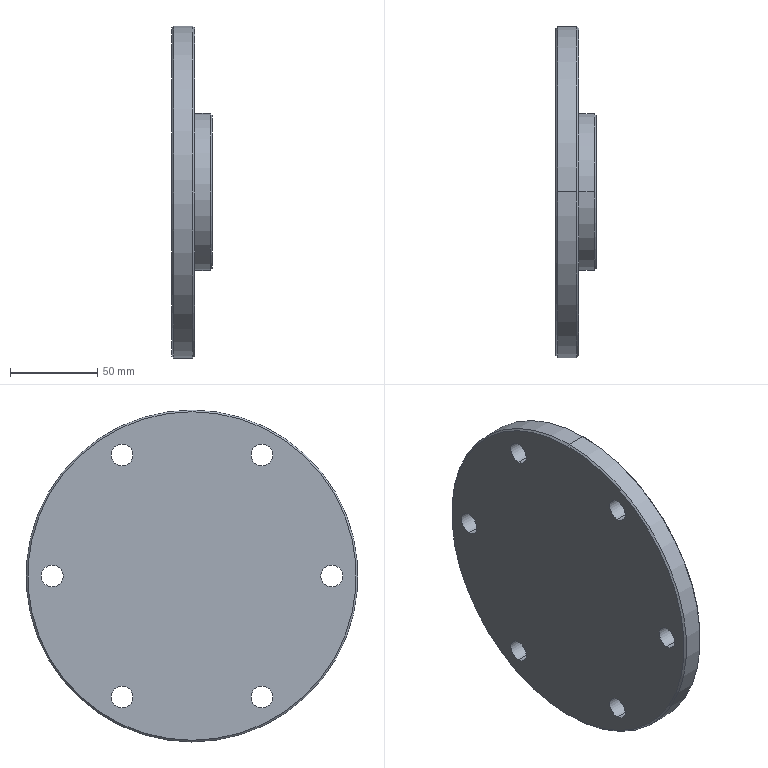Part | SolidWorks | features Chamfer 1, CirPattern 1, ICE 1, Revolution 1 | 1 solid | 30 faces | box 23 x 190 x 190 mm | volume 393528 mm3 | cylinder 18 | cone 8 | plane 4 | commonest cylinder face diameters 12.5 x12 60 x2 90 x2 190 x2
STEP:
#1=CARTESIAN_POINT('',(13.,0.,-94.));
#2=VERTEX_POINT('',#1);
#3=CARTESIAN_POINT('',(13.,0.,94.));
#4=VERTEX_POINT('',#3);
#5=CARTESIAN_POINT('',(13.,0.,0.));
#6=DIRECTION('',(1.,0.,0.));
#7=DIRECTION('',(0.,0.,1.));
#8=AXIS2_PLACEMENT_3D('',#5,#6,#7);
#9=CIRCLE('',#8,94.);
#10=EDGE_CURVE('',#2,#4,#9,.T.);
#11=ORIENTED_EDGE('',*,*,#10,.F.);
#12=CARTESIAN_POINT('',(12.,0.,-95.));
#13=VERTEX_POINT('',#12);
#14=CARTESIAN_POINT('',(12.,0.,-95.));
#15=DIRECTION('',(-0.7071,0.,-0.7071));
#16=VECTOR('',#15,1000.);
#17=LINE('',#14,#16);
#18=EDGE_CURVE('',#2,#13,#17,.T.);
#19=ORIENTED_EDGE('',*,*,#18,.T.);
#20=CARTESIAN_POINT('',(12.,0.,95.));
#21=VERTEX_POINT('',#20);
#22=CARTESIAN_POINT('',(12.,0.,0.));
#23=DIRECTION('',(-1.,0.,0.));
#24=DIRECTION('',(0.,0.,1.));
#25=AXIS2_PLACEMENT_3D('',#22,#23,#24);
#26=CIRCLE('',#25,95.);
#27=EDGE_CURVE('',#21,#13,#26,.T.);
#28=ORIENTED_EDGE('',*,*,#27,.F.);
#29=CARTESIAN_POINT('',(12.,0.,95.));
#30=DIRECTION('',(-0.7071,0.,0.7071));
#31=VECTOR('',#30,1000.);
#32=LINE('',#29,#31);
#33=EDGE_CURVE('',#4,#21,#32,.T.);
#34=ORIENTED_EDGE('',*,*,#33,.F.);
#35=EDGE_LOOP('',(#11,#19,#28,#34));
#36=FACE_OUTER_BOUND('',#35,.T.);
#37=CARTESIAN_POINT('',(12.,0.,0.));
#38=DIRECTION('',(-1.,0.,0.));
#39=DIRECTION('',(0.,0.,1.));
#40=AXIS2_PLACEMENT_3D('',#37,#38,#39);
#41=CONICAL_SURFACE('',#40,95.,0.7854);
#42=ADVANCED_FACE('',(#36),#41,.T.);
#43=CARTESIAN_POINT('',(0.,0.,94.));
#44=VERTEX_POINT('',#43);
#45=CARTESIAN_POINT('',(0.,0.,-94.));
#46=VERTEX_POINT('',#45);
#47=CARTESIAN_POINT('',(0.,0.,0.));
#48=DIRECTION('',(-1.,0.,0.));
#49=DIRECTION('',(0.,0.,-1.));
#50=AXIS2_PLACEMENT_3D('',#47,#48,#49);
#51=CIRCLE('',#50,94.);
#52=EDGE_CURVE('',#44,#46,#51,.T.);
#53=ORIENTED_EDGE('',*,*,#52,.F.);
#54=CARTESIAN_POINT('',(1.,0.,95.));
#55=VERTEX_POINT('',#54);
#56=CARTESIAN_POINT('',(0.,0.,94.));
#57=DIRECTION('',(0.7071,0.,0.7071));
#58=VECTOR('',#57,1000.);
#59=LINE('',#56,#58);
#60=EDGE_CURVE('',#44,#55,#59,.T.);
#61=ORIENTED_EDGE('',*,*,#60,.T.);
#62=CARTESIAN_POINT('',(1.,0.,-95.));
#63=VERTEX_POINT('',#62);
#64=CARTESIAN_POINT('',(1.,0.,0.));
#65=DIRECTION('',(1.,0.,0.));
#66=DIRECTION('',(0.,0.,-1.));
#67=AXIS2_PLACEMENT_3D('',#64,#65,#66);
#68=CIRCLE('',#67,95.);
#69=EDGE_CURVE('',#63,#55,#68,.T.);
#70=ORIENTED_EDGE('',*,*,#69,.F.);
#71=CARTESIAN_POINT('',(0.,0.,-94.));
#72=DIRECTION('',(0.7071,0.,-0.7071));
#73=VECTOR('',#72,1000.);
#74=LINE('',#71,#73);
#75=EDGE_CURVE('',#46,#63,#74,.T.);
#76=ORIENTED_EDGE('',*,*,#75,.F.);
#77=EDGE_LOOP('',(#53,#61,#70,#76));
#78=FACE_OUTER_BOUND('',#77,.T.);
#79=CARTESIAN_POINT('',(0.,0.,0.));
#80=DIRECTION('',(1.,0.,0.));
#81=DIRECTION('',(0.,0.,-1.));
#82=AXIS2_PLACEMENT_3D('',#79,#80,#81);
#83=CONICAL_SURFACE('',#82,94.,0.7854);
#84=ADVANCED_FACE('',(#78),#83,.T.);
#85=CARTESIAN_POINT('',(23.,0.,-44.));
#86=VERTEX_POINT('',#85);
#87=CARTESIAN_POINT('',(23.,0.,44.));
#88=VERTEX_POINT('',#87);
#89=CARTESIAN_POINT('',(23.,0.,0.));
#90=DIRECTION('',(1.,0.,0.));
#91=DIRECTION('',(0.,0.,1.));
#92=AXIS2_PLACEMENT_3D('',#89,#90,#91);
#93=CIRCLE('',#92,44.);
#94=EDGE_CURVE('',#86,#88,#93,.T.);
#95=ORIENTED_EDGE('',*,*,#94,.F.);
#96=CARTESIAN_POINT('',(22.,0.,-45.));
#97=VERTEX_POINT('',#96);
#98=CARTESIAN_POINT('',(22.,0.,-45.));
#99=DIRECTION('',(-0.7071,0.,-0.7071));
#100=VECTOR('',#99,1000.);
#101=LINE('',#98,#100);
#102=EDGE_CURVE('',#86,#97,#101,.T.);
#103=ORIENTED_EDGE('',*,*,#102,.T.);
#104=CARTESIAN_POINT('',(22.,0.,45.));
#105=VERTEX_POINT('',#104);
#106=CARTESIAN_POINT('',(22.,0.,0.));
#107=DIRECTION('',(-1.,0.,0.));
#108=DIRECTION('',(0.,0.,1.));
#109=AXIS2_PLACEMENT_3D('',#106,#107,#108);
#110=CIRCLE('',#109,45.);
#111=EDGE_CURVE('',#105,#97,#110,.T.);
#112=ORIENTED_EDGE('',*,*,#111,.F.);
#113=CARTESIAN_POINT('',(22.,0.,45.));
#114=DIRECTION('',(-0.7071,0.,0.7071));
#115=VECTOR('',#114,1000.);
#116=LINE('',#113,#115);
#117=EDGE_CURVE('',#88,#105,#116,.T.);
#118=ORIENTED_EDGE('',*,*,#117,.F.);
#119=EDGE_LOOP('',(#95,#103,#112,#118));
#120=FACE_OUTER_BOUND('',#119,.T.);
#121=CARTESIAN_POINT('',(22.,0.,0.));
#122=DIRECTION('',(-1.,0.,0.));
#123=DIRECTION('',(0.,0.,1.));
#124=AXIS2_PLACEMENT_3D('',#121,#122,#123);
#125=CONICAL_SURFACE('',#124,45.,0.7854);
#126=ADVANCED_FACE('',(#120),#125,.T.);
#127=CARTESIAN_POINT('',(22.,0.,30.));
#128=VERTEX_POINT('',#127);
#129=CARTESIAN_POINT('',(22.,0.,-30.));
#130=VERTEX_POINT('',#129);
#131=CARTESIAN_POINT('',(22.,0.,0.));
#132=DIRECTION('',(1.,0.,0.));
#133=DIRECTION('',(0.,0.,1.));
#134=AXIS2_PLACEMENT_3D('',#131,#132,#133);
#135=CIRCLE('',#134,30.);
#136=EDGE_CURVE('',#128,#130,#135,.T.);
#137=ORIENTED_EDGE('',*,*,#136,.F.);
#138=CARTESIAN_POINT('',(23.,0.,31.));
#139=VERTEX_POINT('',#138);
#140=CARTESIAN_POINT('',(23.,0.,31.));
#141=DIRECTION('',(0.7071,0.,0.7071));
#142=VECTOR('',#141,1000.);
#143=LINE('',#140,#142);
#144=EDGE_CURVE('',#128,#139,#143,.T.);
#145=ORIENTED_EDGE('',*,*,#144,.T.);
#146=CARTESIAN_POINT('',(23.,0.,-31.));
#147=VERTEX_POINT('',#146);
#148=CARTESIAN_POINT('',(23.,0.,0.));
#149=DIRECTION('',(-1.,0.,0.));
#150=DIRECTION('',(0.,0.,1.));
#151=AXIS2_PLACEMENT_3D('',#148,#149,#150);
#152=CIRCLE('',#151,31.);
#153=EDGE_CURVE('',#147,#139,#152,.T.);
#154=ORIENTED_EDGE('',*,*,#153,.F.);
#155=CARTESIAN_POINT('',(23.,0.,-31.));
#156=DIRECTION('',(0.7071,0.,-0.7071));
#157=VECTOR('',#156,1000.);
#158=LINE('',#155,#157);
#159=EDGE_CURVE('',#130,#147,#158,.T.);
#160=ORIENTED_EDGE('',*,*,#159,.F.);
#161=EDGE_LOOP('',(#137,#145,#154,#160));
#162=FACE_OUTER_BOUND('',#161,.T.);
#163=CARTESIAN_POINT('',(23.,0.,0.));
#164=DIRECTION('',(1.,0.,0.));
#165=DIRECTION('',(0.,0.,-1.));
#166=AXIS2_PLACEMENT_3D('',#163,#164,#165);
#167=CONICAL_SURFACE('',#166,31.,0.7854);
#168=ADVANCED_FACE('',(#162),#167,.F.);
#169=CARTESIAN_POINT('',(13.,-40.,-75.532));
#170=VERTEX_POINT('',#169);
#171=CARTESIAN_POINT('',(13.,-40.,-63.032));
#172=VERTEX_POINT('',#171);
#173=CARTESIAN_POINT('',(13.,-40.,-69.282));
#174=DIRECTION('',(-1.,0.,0.));
#175=DIRECTION('',(0.,0.,1.));
#176=AXIS2_PLACEMENT_3D('',#173,#174,#175);
#177=CIRCLE('',#176,6.25);
#178=EDGE_CURVE('',#170,#172,#177,.T.);
#179=ORIENTED_EDGE('',*,*,#178,.F.);
#180=CARTESIAN_POINT('',(0.,-40.,-75.532));
#181=VERTEX_POINT('',#180);
#182=CARTESIAN_POINT('',(23.,-40.,-75.532));
#183=DIRECTION('',(-1.,0.,0.));
#184=VECTOR('',#183,1000.);
#185=LINE('',#182,#184);
#186=EDGE_CURVE('',#170,#181,#185,.T.);
#187=ORIENTED_EDGE('',*,*,#186,.T.);
#188=CARTESIAN_POINT('',(0.,-40.,-63.032));
#189=VERTEX_POINT('',#188);
#190=CARTESIAN_POINT('',(0.,-40.,-69.282));
#191=DIRECTION('',(-1.,0.,0.));
#192=DIRECTION('',(0.,0.866,-0.5));
#193=AXIS2_PLACEMENT_3D('',#190,#191,#192);
#194=CIRCLE('',#193,6.25);
#195=EDGE_CURVE('',#181,#189,#194,.T.);
#196=ORIENTED_EDGE('',*,*,#195,.T.);
#197=CARTESIAN_POINT('',(23.,-40.,-63.032));
#198=DIRECTION('',(-1.,0.,0.));
#199=VECTOR('',#198,1000.);
#200=LINE('',#197,#199);
#201=EDGE_CURVE('',#172,#189,#200,.T.);
#202=ORIENTED_EDGE('',*,*,#201,.F.);
#203=EDGE_LOOP('',(#179,#187,#196,#202));
#204=FACE_OUTER_BOUND('',#203,.T.);
#205=CARTESIAN_POINT('',(23.,-40.,-69.282));
#206=DIRECTION('',(-1.,0.,0.));
#207=DIRECTION('',(0.,0.,1.));
#208=AXIS2_PLACEMENT_3D('',#205,#206,#207);
#209=CYLINDRICAL_SURFACE('',#208,6.25);
#210=ADVANCED_FACE('',(#204),#209,.F.);
#211=CARTESIAN_POINT('',(13.,-80.,-6.25));
#212=VERTEX_POINT('',#211);
#213=CARTESIAN_POINT('',(13.,-80.,6.25));
#214=VERTEX_POINT('',#213);
#215=CARTESIAN_POINT('',(13.,-80.,0.));
#216=DIRECTION('',(-1.,0.,0.));
#217=DIRECTION('',(0.,0.,1.));
#218=AXIS2_PLACEMENT_3D('',#215,#216,#217);
#219=CIRCLE('',#218,6.25);
#220=EDGE_CURVE('',#212,#214,#219,.T.);
#221=ORIENTED_EDGE('',*,*,#220,.F.);
#222=CARTESIAN_POINT('',(0.,-80.,-6.25));
#223=VERTEX_POINT('',#222);
#224=CARTESIAN_POINT('',(23.,-80.,-6.25));
#225=DIRECTION('',(-1.,0.,0.));
#226=VECTOR('',#225,1000.);
#227=LINE('',#224,#226);
#228=EDGE_CURVE('',#212,#223,#227,.T.);
#229=ORIENTED_EDGE('',*,*,#228,.T.);
#230=CARTESIAN_POINT('',(0.,-80.,6.25));
#231=VERTEX_POINT('',#230);
#232=CARTESIAN_POINT('',(0.,-80.,0.));
#233=DIRECTION('',(-1.,0.,0.));
#234=DIRECTION('',(0.,0.,-1.));
#235=AXIS2_PLACEMENT_3D('',#232,#233,#234);
#236=CIRCLE('',#235,6.25);
#237=EDGE_CURVE('',#223,#231,#236,.T.);
#238=ORIENTED_EDGE('',*,*,#237,.T.);
#239=CARTESIAN_POINT('',(23.,-80.,6.25));
#240=DIRECTION('',(-1.,0.,0.));
#241=VECTOR('',#240,1000.);
#242=LINE('',#239,#241);
#243=EDGE_CURVE('',#214,#231,#242,.T.);
#244=ORIENTED_EDGE('',*,*,#243,.F.);
#245=EDGE_LOOP('',(#221,#229,#238,#244));
#246=FACE_OUTER_BOUND('',#245,.T.);
#247=CARTESIAN_POINT('',(23.,-80.,0.));
#248=DIRECTION('',(-1.,0.,0.));
#249=DIRECTION('',(0.,0.,1.));
#250=AXIS2_PLACEMENT_3D('',#247,#248,#249);
#251=CYLINDRICAL_SURFACE('',#250,6.25);
#252=ADVANCED_FACE('',(#246),#251,.F.);
#253=CARTESIAN_POINT('',(13.,-40.,63.032));
#254=VERTEX_POINT('',#253);
#255=CARTESIAN_POINT('',(13.,-40.,75.532));
#256=VERTEX_POINT('',#255);
#257=CARTESIAN_POINT('',(13.,-40.,69.282));
#258=DIRECTION('',(-1.,0.,0.));
#259=DIRECTION('',(0.,0.,1.));
#260=AXIS2_PLACEMENT_3D('',#257,#258,#259);
#261=CIRCLE('',#260,6.25);
#262=EDGE_CURVE('',#254,#256,#261,.T.);
#263=ORIENTED_EDGE('',*,*,#262,.F.);
#264=CARTESIAN_POINT('',(0.,-40.,63.032));
#265=VERTEX_POINT('',#264);
#266=CARTESIAN_POINT('',(23.,-40.,63.032));
#267=DIRECTION('',(-1.,0.,0.));
#268=VECTOR('',#267,1000.);
#269=LINE('',#266,#268);
#270=EDGE_CURVE('',#254,#265,#269,.T.);
#271=ORIENTED_EDGE('',*,*,#270,.T.);
#272=CARTESIAN_POINT('',(0.,-40.,75.532));
#273=VERTEX_POINT('',#272);
#274=CARTESIAN_POINT('',(0.,-40.,69.282));
#275=DIRECTION('',(-1.,0.,0.));
#276=DIRECTION('',(0.,-0.866,-0.5));
#277=AXIS2_PLACEMENT_3D('',#274,#275,#276);
#278=CIRCLE('',#277,6.25);
#279=EDGE_CURVE('',#265,#273,#278,.T.);
#280=ORIENTED_EDGE('',*,*,#279,.T.);
#281=CARTESIAN_POINT('',(23.,-40.,75.532));
#282=DIRECTION('',(-1.,0.,0.));
#283=VECTOR('',#282,1000.);
#284=LINE('',#281,#283);
#285=EDGE_CURVE('',#256,#273,#284,.T.);
#286=ORIENTED_EDGE('',*,*,#285,.F.);
#287=EDGE_LOOP('',(#263,#271,#280,#286));
#288=FACE_OUTER_BOUND('',#287,.T.);
#289=CARTESIAN_POINT('',(23.,-40.,69.282));
#290=DIRECTION('',(-1.,0.,0.));
#291=DIRECTION('',(0.,0.,1.));
#292=AXIS2_PLACEMENT_3D('',#289,#290,#291);
#293=CYLINDRICAL_SURFACE('',#292,6.25);
#294=ADVANCED_FACE('',(#288),#293,.F.);
#295=CARTESIAN_POINT('',(13.,40.,63.032));
#296=VERTEX_POINT('',#295);
#297=CARTESIAN_POINT('',(13.,40.,75.532));
#298=VERTEX_POINT('',#297);
#299=CARTESIAN_POINT('',(13.,40.,69.282));
#300=DIRECTION('',(-1.,0.,0.));
#301=DIRECTION('',(0.,0.,1.));
#302=AXIS2_PLACEMENT_3D('',#299,#300,#301);
#303=CIRCLE('',#302,6.25);
#304=EDGE_CURVE('',#296,#298,#303,.T.);
#305=ORIENTED_EDGE('',*,*,#304,.F.);
#306=CARTESIAN_POINT('',(0.,40.,63.032));
#307=VERTEX_POINT('',#306);
#308=CARTESIAN_POINT('',(23.,40.,63.032));
#309=DIRECTION('',(-1.,0.,0.));
#310=VECTOR('',#309,1000.);
#311=LINE('',#308,#310);
#312=EDGE_CURVE('',#296,#307,#311,.T.);
#313=ORIENTED_EDGE('',*,*,#312,.T.);
#314=CARTESIAN_POINT('',(0.,40.,75.532));
#315=VERTEX_POINT('',#314);
#316=CARTESIAN_POINT('',(0.,40.,69.282));
#317=DIRECTION('',(-1.,0.,0.));
#318=DIRECTION('',(0.,-0.866,0.5));
#319=AXIS2_PLACEMENT_3D('',#316,#317,#318);
#320=CIRCLE('',#319,6.25);
#321=EDGE_CURVE('',#307,#315,#320,.T.);
#322=ORIENTED_EDGE('',*,*,#321,.T.);
#323=CARTESIAN_POINT('',(23.,40.,75.532));
#324=DIRECTION('',(-1.,0.,0.));
#325=VECTOR('',#324,1000.);
#326=LINE('',#323,#325);
#327=EDGE_CURVE('',#298,#315,#326,.T.);
#328=ORIENTED_EDGE('',*,*,#327,.F.);
#329=EDGE_LOOP('',(#305,#313,#322,#328));
#330=FACE_OUTER_BOUND('',#329,.T.);
#331=CARTESIAN_POINT('',(23.,40.,69.282));
#332=DIRECTION('',(-1.,0.,0.));
#333=DIRECTION('',(0.,0.,1.));
#334=AXIS2_PLACEMENT_3D('',#331,#332,#333);
#335=CYLINDRICAL_SURFACE('',#334,6.25);
#336=ADVANCED_FACE('',(#330),#335,.F.);
#337=CARTESIAN_POINT('',(13.,40.,-75.532));
#338=VERTEX_POINT('',#337);
#339=CARTESIAN_POINT('',(13.,40.,-63.032));
#340=VERTEX_POINT('',#339);
#341=CARTESIAN_POINT('',(13.,40.,-69.282));
#342=DIRECTION('',(-1.,0.,0.));
#343=DIRECTION('',(0.,0.,1.));
#344=AXIS2_PLACEMENT_3D('',#341,#342,#343);
#345=CIRCLE('',#344,6.25);
#346=EDGE_CURVE('',#338,#340,#345,.T.);
#347=ORIENTED_EDGE('',*,*,#346,.F.);
#348=CARTESIAN_POINT('',(0.,40.,-75.532));
#349=VERTEX_POINT('',#348);
#350=CARTESIAN_POINT('',(23.,40.,-75.532));
#351=DIRECTION('',(-1.,0.,0.));
#352=VECTOR('',#351,1000.);
#353=LINE('',#350,#352);
#354=EDGE_CURVE('',#338,#349,#353,.T.);
#355=ORIENTED_EDGE('',*,*,#354,.T.);
#356=CARTESIAN_POINT('',(0.,40.,-63.032));
#357=VERTEX_POINT('',#356);
#358=CARTESIAN_POINT('',(0.,40.,-69.282));
#359=DIRECTION('',(-1.,0.,0.));
#360=DIRECTION('',(0.,0.866,0.5));
#361=AXIS2_PLACEMENT_3D('',#358,#359,#360);
#362=CIRCLE('',#361,6.25);
#363=EDGE_CURVE('',#349,#357,#362,.T.);
#364=ORIENTED_EDGE('',*,*,#363,.T.);
#365=CARTESIAN_POINT('',(23.,40.,-63.032));
#366=DIRECTION('',(-1.,0.,0.));
#367=VECTOR('',#366,1000.);
#368=LINE('',#365,#367);
#369=EDGE_CURVE('',#340,#357,#368,.T.);
#370=ORIENTED_EDGE('',*,*,#369,.F.);
#371=EDGE_LOOP('',(#347,#355,#364,#370));
#372=FACE_OUTER_BOUND('',#371,.T.);
#373=CARTESIAN_POINT('',(23.,40.,-69.282));
#374=DIRECTION('',(-1.,0.,0.));
#375=DIRECTION('',(0.,0.,1.));
#376=AXIS2_PLACEMENT_3D('',#373,#374,#375);
#377=CYLINDRICAL_SURFACE('',#376,6.25);
#378=ADVANCED_FACE('',(#372),#377,.F.);
#379=CARTESIAN_POINT('',(13.,80.,-6.25));
#380=VERTEX_POINT('',#379);
#381=CARTESIAN_POINT('',(13.,80.,6.25));
#382=VERTEX_POINT('',#381);
#383=CARTESIAN_POINT('',(13.,80.,0.));
#384=DIRECTION('',(-1.,0.,0.));
#385=DIRECTION('',(0.,0.,1.));
#386=AXIS2_PLACEMENT_3D('',#383,#384,#385);
#387=CIRCLE('',#386,6.25);
#388=EDGE_CURVE('',#380,#382,#387,.T.);
#389=ORIENTED_EDGE('',*,*,#388,.F.);
#390=CARTESIAN_POINT('',(0.,80.,-6.25));
#391=VERTEX_POINT('',#390);
#392=CARTESIAN_POINT('',(23.,80.,-6.25));
#393=DIRECTION('',(-1.,0.,0.));
#394=VECTOR('',#393,1000.);
#395=LINE('',#392,#394);
#396=EDGE_CURVE('',#380,#391,#395,.T.);
#397=ORIENTED_EDGE('',*,*,#396,.T.);
#398=CARTESIAN_POINT('',(0.,80.,6.25));
#399=VERTEX_POINT('',#398);
#400=CARTESIAN_POINT('',(0.,80.,0.));
#401=DIRECTION('',(-1.,0.,0.));
#402=DIRECTION('',(0.,0.,1.));
#403=AXIS2_PLACEMENT_3D('',#400,#401,#402);
#404=CIRCLE('',#403,6.25);
#405=EDGE_CURVE('',#391,#399,#404,.T.);
#406=ORIENTED_EDGE('',*,*,#405,.T.);
#407=CARTESIAN_POINT('',(23.,80.,6.25));
#408=DIRECTION('',(-1.,0.,0.));
#409=VECTOR('',#408,1000.);
#410=LINE('',#407,#409);
#411=EDGE_CURVE('',#382,#399,#410,.T.);
#412=ORIENTED_EDGE('',*,*,#411,.F.);
#413=EDGE_LOOP('',(#389,#397,#406,#412));
#414=FACE_OUTER_BOUND('',#413,.T.);
#415=CARTESIAN_POINT('',(23.,80.,0.));
#416=DIRECTION('',(-1.,0.,0.));
#417=DIRECTION('',(0.,0.,1.));
#418=AXIS2_PLACEMENT_3D('',#415,#416,#417);
#419=CYLINDRICAL_SURFACE('',#418,6.25);
#420=ADVANCED_FACE('',(#414),#419,.F.);
#421=ORIENTED_EDGE('',*,*,#136,.T.);
#422=CARTESIAN_POINT('',(13.,0.,-30.));
#423=VERTEX_POINT('',#422);
#424=CARTESIAN_POINT('',(0.,0.,-30.));
#425=DIRECTION('',(-1.,0.,0.));
#426=VECTOR('',#425,1000.);
#427=LINE('',#424,#426);
#428=EDGE_CURVE('',#130,#423,#427,.T.);
#429=ORIENTED_EDGE('',*,*,#428,.T.);
#430=CARTESIAN_POINT('',(13.,0.,30.));
#431=VERTEX_POINT('',#430);
#432=CARTESIAN_POINT('',(13.,0.,0.));
#433=DIRECTION('',(-1.,0.,0.));
#434=DIRECTION('',(0.,0.,1.));
#435=AXIS2_PLACEMENT_3D('',#432,#433,#434);
#436=CIRCLE('',#435,30.);
#437=EDGE_CURVE('',#423,#431,#436,.T.);
#438=ORIENTED_EDGE('',*,*,#437,.T.);
#439=CARTESIAN_POINT('',(0.,0.,30.));
#440=DIRECTION('',(-1.,0.,0.));
#441=VECTOR('',#440,1000.);
#442=LINE('',#439,#441);
#443=EDGE_CURVE('',#128,#431,#442,.T.);
#444=ORIENTED_EDGE('',*,*,#443,.F.);
#445=EDGE_LOOP('',(#421,#429,#438,#444));
#446=FACE_OUTER_BOUND('',#445,.T.);
#447=CARTESIAN_POINT('',(0.,0.,0.));
#448=DIRECTION('',(-1.,0.,0.));
#449=DIRECTION('',(0.,0.,1.));
#450=AXIS2_PLACEMENT_3D('',#447,#448,#449);
#451=CYLINDRICAL_SURFACE('',#450,30.);
#452=ADVANCED_FACE('',(#446),#451,.F.);
#453=ORIENTED_EDGE('',*,*,#111,.T.);
#454=CARTESIAN_POINT('',(13.,0.,-45.));
#455=VERTEX_POINT('',#454);
#456=CARTESIAN_POINT('',(0.,0.,-45.));
#457=DIRECTION('',(-1.,0.,0.));
#458=VECTOR('',#457,1000.);
#459=LINE('',#456,#458);
#460=EDGE_CURVE('',#97,#455,#459,.T.);
#461=ORIENTED_EDGE('',*,*,#460,.T.);
#462=CARTESIAN_POINT('',(13.,0.,45.));
#463=VERTEX_POINT('',#462);
#464=CARTESIAN_POINT('',(13.,0.,0.));
#465=DIRECTION('',(-1.,0.,0.));
#466=DIRECTION('',(0.,0.,1.));
#467=AXIS2_PLACEMENT_3D('',#464,#465,#466);
#468=CIRCLE('',#467,45.);
#469=EDGE_CURVE('',#463,#455,#468,.T.);
#470=ORIENTED_EDGE('',*,*,#469,.F.);
#471=CARTESIAN_POINT('',(0.,0.,45.));
#472=DIRECTION('',(-1.,0.,0.));
#473=VECTOR('',#472,1000.);
#474=LINE('',#471,#473);
#475=EDGE_CURVE('',#105,#463,#474,.T.);
#476=ORIENTED_EDGE('',*,*,#475,.F.);
#477=EDGE_LOOP('',(#453,#461,#470,#476));
#478=FACE_OUTER_BOUND('',#477,.T.);
#479=CARTESIAN_POINT('',(0.,0.,0.));
#480=DIRECTION('',(-1.,0.,0.));
#481=DIRECTION('',(0.,0.,1.));
#482=AXIS2_PLACEMENT_3D('',#479,#480,#481);
#483=CYLINDRICAL_SURFACE('',#482,45.);
#484=ADVANCED_FACE('',(#478),#483,.T.);
#485=ORIENTED_EDGE('',*,*,#27,.T.);
#486=CARTESIAN_POINT('',(0.,0.,-95.));
#487=DIRECTION('',(-1.,0.,0.));
#488=VECTOR('',#487,1000.);
#489=LINE('',#486,#488);
#490=EDGE_CURVE('',#13,#63,#489,.T.);
#491=ORIENTED_EDGE('',*,*,#490,.T.);
#492=ORIENTED_EDGE('',*,*,#69,.T.);
#493=CARTESIAN_POINT('',(0.,0.,95.));
#494=DIRECTION('',(-1.,0.,0.));
#495=VECTOR('',#494,1000.);
#496=LINE('',#493,#495);
#497=EDGE_CURVE('',#21,#55,#496,.T.);
#498=ORIENTED_EDGE('',*,*,#497,.F.);
#499=EDGE_LOOP('',(#485,#491,#492,#498));
#500=FACE_OUTER_BOUND('',#499,.T.);
#501=CARTESIAN_POINT('',(0.,0.,0.));
#502=DIRECTION('',(-1.,0.,0.));
#503=DIRECTION('',(0.,0.,1.));
#504=AXIS2_PLACEMENT_3D('',#501,#502,#503);
#505=CYLINDRICAL_SURFACE('',#504,95.);
#506=ADVANCED_FACE('',(#500),#505,.T.);
#507=CARTESIAN_POINT('',(0.,0.,0.));
#508=DIRECTION('',(-1.,0.,0.));
#509=DIRECTION('',(0.,0.,-1.));
#510=AXIS2_PLACEMENT_3D('',#507,#508,#509);
#511=CIRCLE('',#510,94.);
#512=EDGE_CURVE('',#46,#44,#511,.T.);
#513=ORIENTED_EDGE('',*,*,#512,.T.);
#514=ORIENTED_EDGE('',*,*,#52,.T.);
#515=EDGE_LOOP('',(#513,#514));
#516=FACE_OUTER_BOUND('',#515,.T.);
#517=CARTESIAN_POINT('',(0.,-40.,-69.282));
#518=DIRECTION('',(-1.,0.,0.));
#519=DIRECTION('',(0.,0.866,-0.5));
#520=AXIS2_PLACEMENT_3D('',#517,#518,#519);
#521=CIRCLE('',#520,6.25);
#522=EDGE_CURVE('',#189,#181,#521,.T.);
#523=ORIENTED_EDGE('',*,*,#522,.F.);
#524=ORIENTED_EDGE('',*,*,#195,.F.);
#525=EDGE_LOOP('',(#523,#524));
#526=FACE_BOUND('',#525,.T.);
#527=CARTESIAN_POINT('',(0.,-80.,0.));
#528=DIRECTION('',(-1.,0.,0.));
#529=DIRECTION('',(0.,0.,-1.));
#530=AXIS2_PLACEMENT_3D('',#527,#528,#529);
#531=CIRCLE('',#530,6.25);
#532=EDGE_CURVE('',#231,#223,#531,.T.);
#533=ORIENTED_EDGE('',*,*,#532,.F.);
#534=ORIENTED_EDGE('',*,*,#237,.F.);
#535=EDGE_LOOP('',(#533,#534));
#536=FACE_BOUND('',#535,.T.);
#537=CARTESIAN_POINT('',(0.,-40.,69.282));
#538=DIRECTION('',(-1.,0.,0.));
#539=DIRECTION('',(0.,-0.866,-0.5));
#540=AXIS2_PLACEMENT_3D('',#537,#538,#539);
#541=CIRCLE('',#540,6.25);
#542=EDGE_CURVE('',#273,#265,#541,.T.);
#543=ORIENTED_EDGE('',*,*,#542,.F.);
#544=ORIENTED_EDGE('',*,*,#279,.F.);
#545=EDGE_LOOP('',(#543,#544));
#546=FACE_BOUND('',#545,.T.);
#547=CARTESIAN_POINT('',(0.,40.,69.282));
#548=DIRECTION('',(-1.,0.,0.));
#549=DIRECTION('',(0.,-0.866,0.5));
#550=AXIS2_PLACEMENT_3D('',#547,#548,#549);
#551=CIRCLE('',#550,6.25);
#552=EDGE_CURVE('',#315,#307,#551,.T.);
#553=ORIENTED_EDGE('',*,*,#552,.F.);
#554=ORIENTED_EDGE('',*,*,#321,.F.);
#555=EDGE_LOOP('',(#553,#554));
#556=FACE_BOUND('',#555,.T.);
#557=CARTESIAN_POINT('',(0.,40.,-69.282));
#558=DIRECTION('',(-1.,0.,0.));
#559=DIRECTION('',(0.,0.866,0.5));
#560=AXIS2_PLACEMENT_3D('',#557,#558,#559);
#561=CIRCLE('',#560,6.25);
#562=EDGE_CURVE('',#357,#349,#561,.T.);
#563=ORIENTED_EDGE('',*,*,#562,.F.);
#564=ORIENTED_EDGE('',*,*,#363,.F.);
#565=EDGE_LOOP('',(#563,#564));
#566=FACE_BOUND('',#565,.T.);
#567=CARTESIAN_POINT('',(0.,80.,0.));
#568=DIRECTION('',(-1.,0.,0.));
#569=DIRECTION('',(0.,0.,1.));
#570=AXIS2_PLACEMENT_3D('',#567,#568,#569);
#571=CIRCLE('',#570,6.25);
#572=EDGE_CURVE('',#399,#391,#571,.T.);
#573=ORIENTED_EDGE('',*,*,#572,.F.);
#574=ORIENTED_EDGE('',*,*,#405,.F.);
#575=EDGE_LOOP('',(#573,#574));
#576=FACE_BOUND('',#575,.T.);
#577=CARTESIAN_POINT('',(0.,0.,0.));
#578=DIRECTION('',(1.,0.,0.));
#579=DIRECTION('',(0.,0.,-1.));
#580=AXIS2_PLACEMENT_3D('',#577,#578,#579);
#581=PLANE('',#580);
#582=ADVANCED_FACE('',(#516,#526,#536,#546,#556,#566,#576),#581,.F.);
#583=ORIENTED_EDGE('',*,*,#490,.F.);
#584=CARTESIAN_POINT('',(12.,0.,0.));
#585=DIRECTION('',(-1.,0.,0.));
#586=DIRECTION('',(0.,0.,1.));
#587=AXIS2_PLACEMENT_3D('',#584,#585,#586);
#588=CIRCLE('',#587,95.);
#589=EDGE_CURVE('',#13,#21,#588,.T.);
#590=ORIENTED_EDGE('',*,*,#589,.T.);
#591=ORIENTED_EDGE('',*,*,#497,.T.);
#592=CARTESIAN_POINT('',(1.,0.,0.));
#593=DIRECTION('',(1.,0.,0.));
#594=DIRECTION('',(0.,0.,-1.));
#595=AXIS2_PLACEMENT_3D('',#592,#593,#594);
#596=CIRCLE('',#595,95.);
#597=EDGE_CURVE('',#55,#63,#596,.T.);
#598=ORIENTED_EDGE('',*,*,#597,.T.);
#599=EDGE_LOOP('',(#583,#590,#591,#598));
#600=FACE_OUTER_BOUND('',#599,.T.);
#601=CARTESIAN_POINT('',(0.,0.,0.));
#602=DIRECTION('',(-1.,0.,0.));
#603=DIRECTION('',(0.,0.,1.));
#604=AXIS2_PLACEMENT_3D('',#601,#602,#603);
#605=CYLINDRICAL_SURFACE('',#604,95.);
#606=ADVANCED_FACE('',(#600),#605,.T.);
#607=CARTESIAN_POINT('',(13.,0.,0.));
#608=DIRECTION('',(1.,0.,0.));
#609=DIRECTION('',(0.,0.,1.));
#610=AXIS2_PLACEMENT_3D('',#607,#608,#609);
#611=CIRCLE('',#610,94.);
#612=EDGE_CURVE('',#4,#2,#611,.T.);
#613=ORIENTED_EDGE('',*,*,#612,.T.);
#614=ORIENTED_EDGE('',*,*,#10,.T.);
#615=EDGE_LOOP('',(#613,#614));
#616=FACE_OUTER_BOUND('',#615,.T.);
#617=CARTESIAN_POINT('',(13.,-40.,-69.282));
#618=DIRECTION('',(-1.,0.,0.));
#619=DIRECTION('',(0.,0.,1.));
#620=AXIS2_PLACEMENT_3D('',#617,#618,#619);
#621=CIRCLE('',#620,6.25);
#622=EDGE_CURVE('',#172,#170,#621,.T.);
#623=ORIENTED_EDGE('',*,*,#622,.T.);
#624=ORIENTED_EDGE('',*,*,#178,.T.);
#625=EDGE_LOOP('',(#623,#624));
#626=FACE_BOUND('',#625,.T.);
#627=CARTESIAN_POINT('',(13.,-80.,0.));
#628=DIRECTION('',(-1.,0.,0.));
#629=DIRECTION('',(0.,0.,1.));
#630=AXIS2_PLACEMENT_3D('',#627,#628,#629);
#631=CIRCLE('',#630,6.25);
#632=EDGE_CURVE('',#214,#212,#631,.T.);
#633=ORIENTED_EDGE('',*,*,#632,.T.);
#634=ORIENTED_EDGE('',*,*,#220,.T.);
#635=EDGE_LOOP('',(#633,#634));
#636=FACE_BOUND('',#635,.T.);
#637=CARTESIAN_POINT('',(13.,-40.,69.282));
#638=DIRECTION('',(-1.,0.,0.));
#639=DIRECTION('',(0.,0.,1.));
#640=AXIS2_PLACEMENT_3D('',#637,#638,#639);
#641=CIRCLE('',#640,6.25);
#642=EDGE_CURVE('',#256,#254,#641,.T.);
#643=ORIENTED_EDGE('',*,*,#642,.T.);
#644=ORIENTED_EDGE('',*,*,#262,.T.);
#645=EDGE_LOOP('',(#643,#644));
#646=FACE_BOUND('',#645,.T.);
#647=CARTESIAN_POINT('',(13.,40.,69.282));
#648=DIRECTION('',(-1.,0.,0.));
#649=DIRECTION('',(0.,0.,1.));
#650=AXIS2_PLACEMENT_3D('',#647,#648,#649);
#651=CIRCLE('',#650,6.25);
#652=EDGE_CURVE('',#298,#296,#651,.T.);
#653=ORIENTED_EDGE('',*,*,#652,.T.);
#654=ORIENTED_EDGE('',*,*,#304,.T.);
#655=EDGE_LOOP('',(#653,#654));
#656=FACE_BOUND('',#655,.T.);
#657=CARTESIAN_POINT('',(13.,40.,-69.282));
#658=DIRECTION('',(-1.,0.,0.));
#659=DIRECTION('',(0.,0.,1.));
#660=AXIS2_PLACEMENT_3D('',#657,#658,#659);
#661=CIRCLE('',#660,6.25);
#662=EDGE_CURVE('',#340,#338,#661,.T.);
#663=ORIENTED_EDGE('',*,*,#662,.T.);
#664=ORIENTED_EDGE('',*,*,#346,.T.);
#665=EDGE_LOOP('',(#663,#664));
#666=FACE_BOUND('',#665,.T.);
#667=CARTESIAN_POINT('',(13.,80.,0.));
#668=DIRECTION('',(-1.,0.,0.));
#669=DIRECTION('',(0.,0.,1.));
#670=AXIS2_PLACEMENT_3D('',#667,#668,#669);
#671=CIRCLE('',#670,6.25);
#672=EDGE_CURVE('',#382,#380,#671,.T.);
#673=ORIENTED_EDGE('',*,*,#672,.T.);
#674=ORIENTED_EDGE('',*,*,#388,.T.);
#675=EDGE_LOOP('',(#673,#674));
#676=FACE_BOUND('',#675,.T.);
#677=ORIENTED_EDGE('',*,*,#469,.T.);
#678=CARTESIAN_POINT('',(13.,0.,0.));
#679=DIRECTION('',(-1.,0.,0.));
#680=DIRECTION('',(0.,0.,1.));
#681=AXIS2_PLACEMENT_3D('',#678,#679,#680);
#682=CIRCLE('',#681,45.);
#683=EDGE_CURVE('',#455,#463,#682,.T.);
#684=ORIENTED_EDGE('',*,*,#683,.T.);
#685=EDGE_LOOP('',(#677,#684));
#686=FACE_BOUND('',#685,.T.);
#687=CARTESIAN_POINT('',(13.,95.,0.));
#688=DIRECTION('',(-1.,0.,0.));
#689=DIRECTION('',(0.,0.,1.));
#690=AXIS2_PLACEMENT_3D('',#687,#688,#689);
#691=PLANE('',#690);
#692=ADVANCED_FACE('',(#616,#626,#636,#646,#656,#666,#676,#686),#691,.F.);
#693=ORIENTED_EDGE('',*,*,#460,.F.);
#694=CARTESIAN_POINT('',(22.,0.,0.));
#695=DIRECTION('',(-1.,0.,0.));
#696=DIRECTION('',(0.,0.,1.));
#697=AXIS2_PLACEMENT_3D('',#694,#695,#696);
#698=CIRCLE('',#697,45.);
#699=EDGE_CURVE('',#97,#105,#698,.T.);
#700=ORIENTED_EDGE('',*,*,#699,.T.);
#701=ORIENTED_EDGE('',*,*,#475,.T.);
#702=ORIENTED_EDGE('',*,*,#683,.F.);
#703=EDGE_LOOP('',(#693,#700,#701,#702));
#704=FACE_OUTER_BOUND('',#703,.T.);
#705=CARTESIAN_POINT('',(0.,0.,0.));
#706=DIRECTION('',(-1.,0.,0.));
#707=DIRECTION('',(0.,0.,1.));
#708=AXIS2_PLACEMENT_3D('',#705,#706,#707);
#709=CYLINDRICAL_SURFACE('',#708,45.);
#710=ADVANCED_FACE('',(#704),#709,.T.);
#711=ORIENTED_EDGE('',*,*,#153,.T.);
#712=CARTESIAN_POINT('',(23.,0.,0.));
#713=DIRECTION('',(-1.,0.,0.));
#714=DIRECTION('',(0.,0.,1.));
#715=AXIS2_PLACEMENT_3D('',#712,#713,#714);
#716=CIRCLE('',#715,31.);
#717=EDGE_CURVE('',#139,#147,#716,.T.);
#718=ORIENTED_EDGE('',*,*,#717,.T.);
#719=EDGE_LOOP('',(#711,#718));
#720=FACE_BOUND('',#719,.T.);
#721=CARTESIAN_POINT('',(23.,0.,0.));
#722=DIRECTION('',(1.,0.,0.));
#723=DIRECTION('',(0.,0.,1.));
#724=AXIS2_PLACEMENT_3D('',#721,#722,#723);
#725=CIRCLE('',#724,44.);
#726=EDGE_CURVE('',#88,#86,#725,.T.);
#727=ORIENTED_EDGE('',*,*,#726,.T.);
#728=ORIENTED_EDGE('',*,*,#94,.T.);
#729=EDGE_LOOP('',(#727,#728));
#730=FACE_OUTER_BOUND('',#729,.T.);
#731=CARTESIAN_POINT('',(23.,45.,0.));
#732=DIRECTION('',(-1.,0.,0.));
#733=DIRECTION('',(0.,0.,1.));
#734=AXIS2_PLACEMENT_3D('',#731,#732,#733);
#735=PLANE('',#734);
#736=ADVANCED_FACE('',(#720,#730),#735,.F.);
#737=ORIENTED_EDGE('',*,*,#428,.F.);
#738=CARTESIAN_POINT('',(22.,0.,0.));
#739=DIRECTION('',(1.,0.,0.));
#740=DIRECTION('',(0.,0.,1.));
#741=AXIS2_PLACEMENT_3D('',#738,#739,#740);
#742=CIRCLE('',#741,30.);
#743=EDGE_CURVE('',#130,#128,#742,.T.);
#744=ORIENTED_EDGE('',*,*,#743,.T.);
#745=ORIENTED_EDGE('',*,*,#443,.T.);
#746=CARTESIAN_POINT('',(13.,0.,0.));
#747=DIRECTION('',(-1.,0.,0.));
#748=DIRECTION('',(0.,0.,1.));
#749=AXIS2_PLACEMENT_3D('',#746,#747,#748);
#750=CIRCLE('',#749,30.);
#751=EDGE_CURVE('',#431,#423,#750,.T.);
#752=ORIENTED_EDGE('',*,*,#751,.T.);
#753=EDGE_LOOP('',(#737,#744,#745,#752));
#754=FACE_OUTER_BOUND('',#753,.T.);
#755=CARTESIAN_POINT('',(0.,0.,0.));
#756=DIRECTION('',(-1.,0.,0.));
#757=DIRECTION('',(0.,0.,1.));
#758=AXIS2_PLACEMENT_3D('',#755,#756,#757);
#759=CYLINDRICAL_SURFACE('',#758,30.);
#760=ADVANCED_FACE('',(#754),#759,.F.);
#761=ORIENTED_EDGE('',*,*,#751,.F.);
#762=ORIENTED_EDGE('',*,*,#437,.F.);
#763=EDGE_LOOP('',(#761,#762));
#764=FACE_OUTER_BOUND('',#763,.T.);
#765=CARTESIAN_POINT('',(13.,30.,0.));
#766=DIRECTION('',(-1.,0.,0.));
#767=DIRECTION('',(0.,0.,1.));
#768=AXIS2_PLACEMENT_3D('',#765,#766,#767);
#769=PLANE('',#768);
#770=ADVANCED_FACE('',(#764),#769,.F.);
#771=ORIENTED_EDGE('',*,*,#396,.F.);
#772=ORIENTED_EDGE('',*,*,#672,.F.);
#773=ORIENTED_EDGE('',*,*,#411,.T.);
#774=ORIENTED_EDGE('',*,*,#572,.T.);
#775=EDGE_LOOP('',(#771,#772,#773,#774));
#776=FACE_OUTER_BOUND('',#775,.T.);
#777=CARTESIAN_POINT('',(23.,80.,0.));
#778=DIRECTION('',(-1.,0.,0.));
#779=DIRECTION('',(0.,0.,1.));
#780=AXIS2_PLACEMENT_3D('',#777,#778,#779);
#781=CYLINDRICAL_SURFACE('',#780,6.25);
#782=ADVANCED_FACE('',(#776),#781,.F.);
#783=ORIENTED_EDGE('',*,*,#354,.F.);
#784=ORIENTED_EDGE('',*,*,#662,.F.);
#785=ORIENTED_EDGE('',*,*,#369,.T.);
#786=ORIENTED_EDGE('',*,*,#562,.T.);
#787=EDGE_LOOP('',(#783,#784,#785,#786));
#788=FACE_OUTER_BOUND('',#787,.T.);
#789=CARTESIAN_POINT('',(23.,40.,-69.282));
#790=DIRECTION('',(-1.,0.,0.));
#791=DIRECTION('',(0.,0.,1.));
#792=AXIS2_PLACEMENT_3D('',#789,#790,#791);
#793=CYLINDRICAL_SURFACE('',#792,6.25);
#794=ADVANCED_FACE('',(#788),#793,.F.);
#795=ORIENTED_EDGE('',*,*,#312,.F.);
#796=ORIENTED_EDGE('',*,*,#652,.F.);
#797=ORIENTED_EDGE('',*,*,#327,.T.);
#798=ORIENTED_EDGE('',*,*,#552,.T.);
#799=EDGE_LOOP('',(#795,#796,#797,#798));
#800=FACE_OUTER_BOUND('',#799,.T.);
#801=CARTESIAN_POINT('',(23.,40.,69.282));
#802=DIRECTION('',(-1.,0.,0.));
#803=DIRECTION('',(0.,0.,1.));
#804=AXIS2_PLACEMENT_3D('',#801,#802,#803);
#805=CYLINDRICAL_SURFACE('',#804,6.25);
#806=ADVANCED_FACE('',(#800),#805,.F.);
#807=ORIENTED_EDGE('',*,*,#270,.F.);
#808=ORIENTED_EDGE('',*,*,#642,.F.);
#809=ORIENTED_EDGE('',*,*,#285,.T.);
#810=ORIENTED_EDGE('',*,*,#542,.T.);
#811=EDGE_LOOP('',(#807,#808,#809,#810));
#812=FACE_OUTER_BOUND('',#811,.T.);
#813=CARTESIAN_POINT('',(23.,-40.,69.282));
#814=DIRECTION('',(-1.,0.,0.));
#815=DIRECTION('',(0.,0.,1.));
#816=AXIS2_PLACEMENT_3D('',#813,#814,#815);
#817=CYLINDRICAL_SURFACE('',#816,6.25);
#818=ADVANCED_FACE('',(#812),#817,.F.);
#819=ORIENTED_EDGE('',*,*,#228,.F.);
#820=ORIENTED_EDGE('',*,*,#632,.F.);
#821=ORIENTED_EDGE('',*,*,#243,.T.);
#822=ORIENTED_EDGE('',*,*,#532,.T.);
#823=EDGE_LOOP('',(#819,#820,#821,#822));
#824=FACE_OUTER_BOUND('',#823,.T.);
#825=CARTESIAN_POINT('',(23.,-80.,0.));
#826=DIRECTION('',(-1.,0.,0.));
#827=DIRECTION('',(0.,0.,1.));
#828=AXIS2_PLACEMENT_3D('',#825,#826,#827);
#829=CYLINDRICAL_SURFACE('',#828,6.25);
#830=ADVANCED_FACE('',(#824),#829,.F.);
#831=ORIENTED_EDGE('',*,*,#186,.F.);
#832=ORIENTED_EDGE('',*,*,#622,.F.);
#833=ORIENTED_EDGE('',*,*,#201,.T.);
#834=ORIENTED_EDGE('',*,*,#522,.T.);
#835=EDGE_LOOP('',(#831,#832,#833,#834));
#836=FACE_OUTER_BOUND('',#835,.T.);
#837=CARTESIAN_POINT('',(23.,-40.,-69.282));
#838=DIRECTION('',(-1.,0.,0.));
#839=DIRECTION('',(0.,0.,1.));
#840=AXIS2_PLACEMENT_3D('',#837,#838,#839);
#841=CYLINDRICAL_SURFACE('',#840,6.25);
#842=ADVANCED_FACE('',(#836),#841,.F.);
#843=ORIENTED_EDGE('',*,*,#144,.F.);
#844=ORIENTED_EDGE('',*,*,#743,.F.);
#845=ORIENTED_EDGE('',*,*,#159,.T.);
#846=ORIENTED_EDGE('',*,*,#717,.F.);
#847=EDGE_LOOP('',(#843,#844,#845,#846));
#848=FACE_OUTER_BOUND('',#847,.T.);
#849=CARTESIAN_POINT('',(23.,0.,0.));
#850=DIRECTION('',(1.,0.,0.));
#851=DIRECTION('',(0.,0.,-1.));
#852=AXIS2_PLACEMENT_3D('',#849,#850,#851);
#853=CONICAL_SURFACE('',#852,31.,0.7854);
#854=ADVANCED_FACE('',(#848),#853,.F.);
#855=ORIENTED_EDGE('',*,*,#102,.F.);
#856=ORIENTED_EDGE('',*,*,#726,.F.);
#857=ORIENTED_EDGE('',*,*,#117,.T.);
#858=ORIENTED_EDGE('',*,*,#699,.F.);
#859=EDGE_LOOP('',(#855,#856,#857,#858));
#860=FACE_OUTER_BOUND('',#859,.T.);
#861=CARTESIAN_POINT('',(22.,0.,0.));
#862=DIRECTION('',(-1.,0.,0.));
#863=DIRECTION('',(0.,0.,1.));
#864=AXIS2_PLACEMENT_3D('',#861,#862,#863);
#865=CONICAL_SURFACE('',#864,45.,0.7854);
#866=ADVANCED_FACE('',(#860),#865,.T.);
#867=ORIENTED_EDGE('',*,*,#60,.F.);
#868=ORIENTED_EDGE('',*,*,#512,.F.);
#869=ORIENTED_EDGE('',*,*,#75,.T.);
#870=ORIENTED_EDGE('',*,*,#597,.F.);
#871=EDGE_LOOP('',(#867,#868,#869,#870));
#872=FACE_OUTER_BOUND('',#871,.T.);
#873=CARTESIAN_POINT('',(0.,0.,0.));
#874=DIRECTION('',(1.,0.,0.));
#875=DIRECTION('',(0.,0.,-1.));
#876=AXIS2_PLACEMENT_3D('',#873,#874,#875);
#877=CONICAL_SURFACE('',#876,94.,0.7854);
#878=ADVANCED_FACE('',(#872),#877,.T.);
#879=ORIENTED_EDGE('',*,*,#18,.F.);
#880=ORIENTED_EDGE('',*,*,#612,.F.);
#881=ORIENTED_EDGE('',*,*,#33,.T.);
#882=ORIENTED_EDGE('',*,*,#589,.F.);
#883=EDGE_LOOP('',(#879,#880,#881,#882));
#884=FACE_OUTER_BOUND('',#883,.T.);
#885=CARTESIAN_POINT('',(12.,0.,0.));
#886=DIRECTION('',(-1.,0.,0.));
#887=DIRECTION('',(0.,0.,1.));
#888=AXIS2_PLACEMENT_3D('',#885,#886,#887);
#889=CONICAL_SURFACE('',#888,95.,0.7854);
#890=ADVANCED_FACE('',(#884),#889,.T.);
#891=CLOSED_SHELL('',(#42,#84,#126,#168,#210,#252,#294,#336,#378,#420,#452,#484,#506,#582,#606,#692,#710,#736,#760,#770,#782,#794,#806,#818,#830,#842,#854,#866,#878,#890));
#892=MANIFOLD_SOLID_BREP('',#891);
#893=CARTESIAN_POINT('',(0.,0.,0.));
#894=DIRECTION('',(0.,0.,1.));
#895=DIRECTION('',(1.,0.,0.));
#896=AXIS2_PLACEMENT_3D('',#893,#894,#895);
#897=(LENGTH_UNIT()NAMED_UNIT(*)SI_UNIT(.MILLI.,.METRE.));
#898=UNCERTAINTY_MEASURE_WITH_UNIT(LENGTH_MEASURE(0.00001),#897,'','');
#899=(NAMED_UNIT(*)PLANE_ANGLE_UNIT()SI_UNIT($,.RADIAN.));
#900=(NAMED_UNIT(*)SI_UNIT($,.STERADIAN.)SOLID_ANGLE_UNIT());
#901=(GEOMETRIC_REPRESENTATION_CONTEXT(3)GLOBAL_UNCERTAINTY_ASSIGNED_CONTEXT((#898))GLOBAL_UNIT_ASSIGNED_CONTEXT((#897,#899,#900))REPRESENTATION_CONTEXT('',''));
#902=ADVANCED_BREP_SHAPE_REPRESENTATION('',(#892,#896),#901);